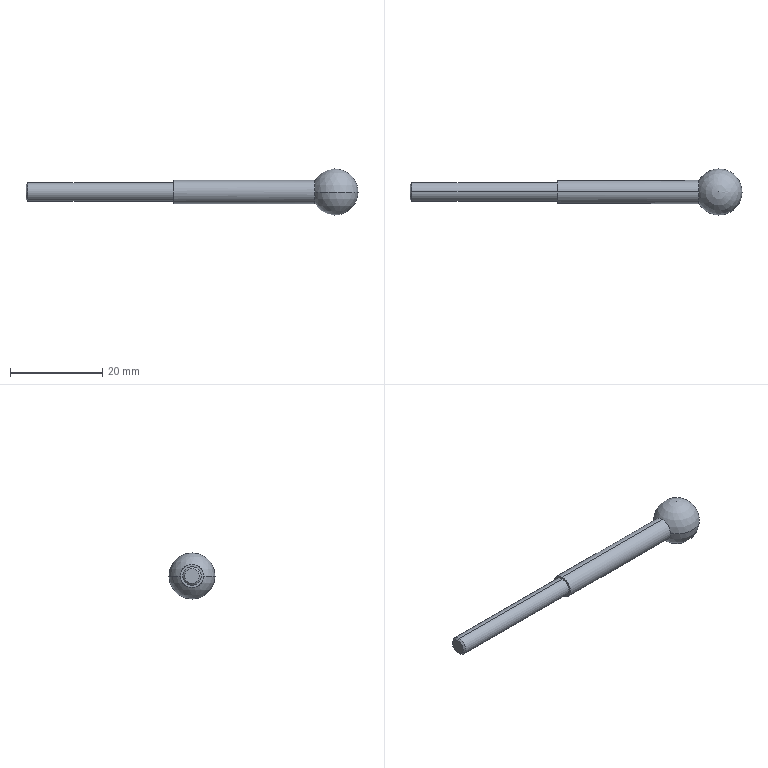Part | SolidWorks | features Extrusion 1, Revolution 1, StudWizard 1 | 1 solid | 10 faces | box 72 x 10 x 10 mm | volume 1520 mm3 | cylinder 4 | sphere 2 | cone 2 | plane 2 | commonest cylinder face diameters 4 x2 5 x2
STEP:
#1=CARTESIAN_POINT('',(67.,-5.,0.));
#2=VERTEX_POINT('',#1);
#3=CARTESIAN_POINT('',(67.,5.,0.));
#4=VERTEX_POINT('',#3);
#5=CARTESIAN_POINT('',(67.,0.,0.));
#6=DIRECTION('',(0.,0.,1.));
#7=DIRECTION('',(1.,0.,0.));
#8=AXIS2_PLACEMENT_3D('',#5,#6,#7);
#9=CIRCLE('',#8,5.);
#10=EDGE_CURVE('',#2,#4,#9,.T.);
#11=ORIENTED_EDGE('',*,*,#10,.F.);
#12=CARTESIAN_POINT('',(62.67,-2.5,0.));
#13=VERTEX_POINT('',#12);
#14=CARTESIAN_POINT('',(67.,0.,0.));
#15=DIRECTION('',(0.,0.,-1.));
#16=DIRECTION('',(-1.,0.,0.));
#17=AXIS2_PLACEMENT_3D('',#14,#15,#16);
#18=CIRCLE('',#17,5.);
#19=EDGE_CURVE('',#2,#13,#18,.T.);
#20=ORIENTED_EDGE('',*,*,#19,.T.);
#21=CARTESIAN_POINT('',(62.67,0.,-2.5));
#22=VERTEX_POINT('',#21);
#23=CARTESIAN_POINT('',(62.67,0.,0.));
#24=DIRECTION('',(1.,0.,0.));
#25=DIRECTION('',(0.,0.,-1.));
#26=AXIS2_PLACEMENT_3D('',#23,#24,#25);
#27=CIRCLE('',#26,2.5);
#28=EDGE_CURVE('',#13,#22,#27,.T.);
#29=ORIENTED_EDGE('',*,*,#28,.T.);
#30=CARTESIAN_POINT('',(62.67,2.5,0.));
#31=VERTEX_POINT('',#30);
#32=CARTESIAN_POINT('',(62.67,0.,0.));
#33=DIRECTION('',(1.,0.,0.));
#34=DIRECTION('',(0.,0.,-1.));
#35=AXIS2_PLACEMENT_3D('',#32,#33,#34);
#36=CIRCLE('',#35,2.5);
#37=EDGE_CURVE('',#22,#31,#36,.T.);
#38=ORIENTED_EDGE('',*,*,#37,.T.);
#39=CARTESIAN_POINT('',(67.,0.,0.));
#40=DIRECTION('',(0.,0.,-1.));
#41=DIRECTION('',(-1.,0.,0.));
#42=AXIS2_PLACEMENT_3D('',#39,#40,#41);
#43=CIRCLE('',#42,5.);
#44=EDGE_CURVE('',#31,#4,#43,.T.);
#45=ORIENTED_EDGE('',*,*,#44,.T.);
#46=EDGE_LOOP('',(#11,#20,#29,#38,#45));
#47=FACE_OUTER_BOUND('',#46,.T.);
#48=CARTESIAN_POINT('',(67.,0.,0.));
#49=DIRECTION('',(0.,0.,-1.));
#50=DIRECTION('',(1.,0.,0.));
#51=AXIS2_PLACEMENT_3D('',#48,#49,#50);
#52=SPHERICAL_SURFACE('',#51,5.);
#53=ADVANCED_FACE('',(#47),#52,.T.);
#54=CARTESIAN_POINT('',(0.,0.,-1.621));
#55=VERTEX_POINT('',#54);
#56=CARTESIAN_POINT('',(0.,0.,1.621));
#57=VERTEX_POINT('',#56);
#58=CARTESIAN_POINT('',(0.,0.,0.));
#59=DIRECTION('',(1.,0.,0.));
#60=DIRECTION('',(0.,0.,-1.));
#61=AXIS2_PLACEMENT_3D('',#58,#59,#60);
#62=CIRCLE('',#61,1.621);
#63=EDGE_CURVE('',#55,#57,#62,.T.);
#64=ORIENTED_EDGE('',*,*,#63,.T.);
#65=CARTESIAN_POINT('',(0.379,0.,2.));
#66=VERTEX_POINT('',#65);
#67=CARTESIAN_POINT('',(0.,0.,1.621));
#68=DIRECTION('',(0.7071,0.,0.7071));
#69=VECTOR('',#68,1000.);
#70=LINE('',#67,#69);
#71=EDGE_CURVE('',#57,#66,#70,.T.);
#72=ORIENTED_EDGE('',*,*,#71,.T.);
#73=CARTESIAN_POINT('',(0.379,0.,-2.));
#74=VERTEX_POINT('',#73);
#75=CARTESIAN_POINT('',(0.379,0.,0.));
#76=DIRECTION('',(1.,0.,0.));
#77=DIRECTION('',(0.,0.,-1.));
#78=AXIS2_PLACEMENT_3D('',#75,#76,#77);
#79=CIRCLE('',#78,2.);
#80=EDGE_CURVE('',#74,#66,#79,.T.);
#81=ORIENTED_EDGE('',*,*,#80,.F.);
#82=CARTESIAN_POINT('',(0.,0.,-1.621));
#83=DIRECTION('',(0.7071,0.,-0.7071));
#84=VECTOR('',#83,1000.);
#85=LINE('',#82,#84);
#86=EDGE_CURVE('',#55,#74,#85,.T.);
#87=ORIENTED_EDGE('',*,*,#86,.F.);
#88=EDGE_LOOP('',(#64,#72,#81,#87));
#89=FACE_OUTER_BOUND('',#88,.T.);
#90=CARTESIAN_POINT('',(0.,0.,0.));
#91=DIRECTION('',(1.,0.,0.));
#92=DIRECTION('',(0.,0.,-1.));
#93=AXIS2_PLACEMENT_3D('',#90,#91,#92);
#94=CONICAL_SURFACE('',#93,1.621,0.7854);
#95=ADVANCED_FACE('',(#89),#94,.T.);
#96=ORIENTED_EDGE('',*,*,#80,.T.);
#97=CARTESIAN_POINT('',(32.,0.,2.));
#98=VERTEX_POINT('',#97);
#99=CARTESIAN_POINT('',(0.,0.,2.));
#100=DIRECTION('',(1.,0.,0.));
#101=VECTOR('',#100,1000.);
#102=LINE('',#99,#101);
#103=EDGE_CURVE('',#66,#98,#102,.T.);
#104=ORIENTED_EDGE('',*,*,#103,.T.);
#105=CARTESIAN_POINT('',(32.,0.,-2.));
#106=VERTEX_POINT('',#105);
#107=CARTESIAN_POINT('',(32.,0.,0.));
#108=DIRECTION('',(1.,0.,0.));
#109=DIRECTION('',(0.,0.,-1.));
#110=AXIS2_PLACEMENT_3D('',#107,#108,#109);
#111=CIRCLE('',#110,2.);
#112=EDGE_CURVE('',#106,#98,#111,.T.);
#113=ORIENTED_EDGE('',*,*,#112,.F.);
#114=CARTESIAN_POINT('',(0.,0.,-2.));
#115=DIRECTION('',(1.,0.,0.));
#116=VECTOR('',#115,1000.);
#117=LINE('',#114,#116);
#118=EDGE_CURVE('',#74,#106,#117,.T.);
#119=ORIENTED_EDGE('',*,*,#118,.F.);
#120=EDGE_LOOP('',(#96,#104,#113,#119));
#121=FACE_OUTER_BOUND('',#120,.T.);
#122=CARTESIAN_POINT('',(0.,0.,0.));
#123=DIRECTION('',(1.,0.,0.));
#124=DIRECTION('',(0.,0.,-1.));
#125=AXIS2_PLACEMENT_3D('',#122,#123,#124);
#126=CYLINDRICAL_SURFACE('',#125,2.);
#127=ADVANCED_FACE('',(#121),#126,.T.);
#128=ORIENTED_EDGE('',*,*,#37,.F.);
#129=CARTESIAN_POINT('',(32.,0.,-2.5));
#130=VERTEX_POINT('',#129);
#131=CARTESIAN_POINT('',(67.,0.,-2.5));
#132=DIRECTION('',(-1.,0.,0.));
#133=VECTOR('',#132,1000.);
#134=LINE('',#131,#133);
#135=EDGE_CURVE('',#22,#130,#134,.T.);
#136=ORIENTED_EDGE('',*,*,#135,.T.);
#137=CARTESIAN_POINT('',(32.,0.,2.5));
#138=VERTEX_POINT('',#137);
#139=CARTESIAN_POINT('',(32.,0.,0.));
#140=DIRECTION('',(1.,0.,0.));
#141=DIRECTION('',(0.,0.,-1.));
#142=AXIS2_PLACEMENT_3D('',#139,#140,#141);
#143=CIRCLE('',#142,2.5);
#144=EDGE_CURVE('',#130,#138,#143,.T.);
#145=ORIENTED_EDGE('',*,*,#144,.T.);
#146=CARTESIAN_POINT('',(62.67,0.,2.5));
#147=VERTEX_POINT('',#146);
#148=CARTESIAN_POINT('',(67.,0.,2.5));
#149=DIRECTION('',(-1.,0.,0.));
#150=VECTOR('',#149,1000.);
#151=LINE('',#148,#150);
#152=EDGE_CURVE('',#147,#138,#151,.T.);
#153=ORIENTED_EDGE('',*,*,#152,.F.);
#154=CARTESIAN_POINT('',(62.67,0.,0.));
#155=DIRECTION('',(1.,0.,0.));
#156=DIRECTION('',(0.,0.,-1.));
#157=AXIS2_PLACEMENT_3D('',#154,#155,#156);
#158=CIRCLE('',#157,2.5);
#159=EDGE_CURVE('',#31,#147,#158,.T.);
#160=ORIENTED_EDGE('',*,*,#159,.F.);
#161=EDGE_LOOP('',(#128,#136,#145,#153,#160));
#162=FACE_OUTER_BOUND('',#161,.T.);
#163=CARTESIAN_POINT('',(67.,0.,0.));
#164=DIRECTION('',(-1.,0.,0.));
#165=DIRECTION('',(0.,0.,1.));
#166=AXIS2_PLACEMENT_3D('',#163,#164,#165);
#167=CYLINDRICAL_SURFACE('',#166,2.5);
#168=ADVANCED_FACE('',(#162),#167,.T.);
#169=ORIENTED_EDGE('',*,*,#135,.F.);
#170=ORIENTED_EDGE('',*,*,#28,.F.);
#171=CARTESIAN_POINT('',(62.67,0.,0.));
#172=DIRECTION('',(1.,0.,0.));
#173=DIRECTION('',(0.,0.,-1.));
#174=AXIS2_PLACEMENT_3D('',#171,#172,#173);
#175=CIRCLE('',#174,2.5);
#176=EDGE_CURVE('',#147,#13,#175,.T.);
#177=ORIENTED_EDGE('',*,*,#176,.F.);
#178=ORIENTED_EDGE('',*,*,#152,.T.);
#179=CARTESIAN_POINT('',(32.,0.,0.));
#180=DIRECTION('',(1.,0.,0.));
#181=DIRECTION('',(0.,0.,-1.));
#182=AXIS2_PLACEMENT_3D('',#179,#180,#181);
#183=CIRCLE('',#182,2.5);
#184=EDGE_CURVE('',#138,#130,#183,.T.);
#185=ORIENTED_EDGE('',*,*,#184,.T.);
#186=EDGE_LOOP('',(#169,#170,#177,#178,#185));
#187=FACE_OUTER_BOUND('',#186,.T.);
#188=CARTESIAN_POINT('',(67.,0.,0.));
#189=DIRECTION('',(-1.,0.,0.));
#190=DIRECTION('',(0.,0.,1.));
#191=AXIS2_PLACEMENT_3D('',#188,#189,#190);
#192=CYLINDRICAL_SURFACE('',#191,2.5);
#193=ADVANCED_FACE('',(#187),#192,.T.);
#194=ORIENTED_EDGE('',*,*,#103,.F.);
#195=CARTESIAN_POINT('',(0.379,0.,0.));
#196=DIRECTION('',(1.,0.,0.));
#197=DIRECTION('',(0.,0.,-1.));
#198=AXIS2_PLACEMENT_3D('',#195,#196,#197);
#199=CIRCLE('',#198,2.);
#200=EDGE_CURVE('',#66,#74,#199,.T.);
#201=ORIENTED_EDGE('',*,*,#200,.T.);
#202=ORIENTED_EDGE('',*,*,#118,.T.);
#203=CARTESIAN_POINT('',(32.,0.,0.));
#204=DIRECTION('',(1.,0.,0.));
#205=DIRECTION('',(0.,0.,-1.));
#206=AXIS2_PLACEMENT_3D('',#203,#204,#205);
#207=CIRCLE('',#206,2.);
#208=EDGE_CURVE('',#98,#106,#207,.T.);
#209=ORIENTED_EDGE('',*,*,#208,.F.);
#210=EDGE_LOOP('',(#194,#201,#202,#209));
#211=FACE_OUTER_BOUND('',#210,.T.);
#212=CARTESIAN_POINT('',(0.,0.,0.));
#213=DIRECTION('',(1.,0.,0.));
#214=DIRECTION('',(0.,0.,-1.));
#215=AXIS2_PLACEMENT_3D('',#212,#213,#214);
#216=CYLINDRICAL_SURFACE('',#215,2.);
#217=ADVANCED_FACE('',(#211),#216,.T.);
#218=ORIENTED_EDGE('',*,*,#184,.F.);
#219=ORIENTED_EDGE('',*,*,#144,.F.);
#220=EDGE_LOOP('',(#218,#219));
#221=FACE_OUTER_BOUND('',#220,.T.);
#222=ORIENTED_EDGE('',*,*,#112,.T.);
#223=ORIENTED_EDGE('',*,*,#208,.T.);
#224=EDGE_LOOP('',(#222,#223));
#225=FACE_BOUND('',#224,.T.);
#226=CARTESIAN_POINT('',(32.,2.,0.));
#227=DIRECTION('',(1.,0.,0.));
#228=DIRECTION('',(0.,0.,-1.));
#229=AXIS2_PLACEMENT_3D('',#226,#227,#228);
#230=PLANE('',#229);
#231=ADVANCED_FACE('',(#221,#225),#230,.F.);
#232=ORIENTED_EDGE('',*,*,#71,.F.);
#233=CARTESIAN_POINT('',(0.,0.,0.));
#234=DIRECTION('',(1.,0.,0.));
#235=DIRECTION('',(0.,0.,-1.));
#236=AXIS2_PLACEMENT_3D('',#233,#234,#235);
#237=CIRCLE('',#236,1.621);
#238=EDGE_CURVE('',#57,#55,#237,.T.);
#239=ORIENTED_EDGE('',*,*,#238,.T.);
#240=ORIENTED_EDGE('',*,*,#86,.T.);
#241=ORIENTED_EDGE('',*,*,#200,.F.);
#242=EDGE_LOOP('',(#232,#239,#240,#241));
#243=FACE_OUTER_BOUND('',#242,.T.);
#244=CARTESIAN_POINT('',(0.,0.,0.));
#245=DIRECTION('',(1.,0.,0.));
#246=DIRECTION('',(0.,0.,-1.));
#247=AXIS2_PLACEMENT_3D('',#244,#245,#246);
#248=CONICAL_SURFACE('',#247,1.621,0.7854);
#249=ADVANCED_FACE('',(#243),#248,.T.);
#250=ORIENTED_EDGE('',*,*,#63,.F.);
#251=ORIENTED_EDGE('',*,*,#238,.F.);
#252=EDGE_LOOP('',(#250,#251));
#253=FACE_OUTER_BOUND('',#252,.T.);
#254=CARTESIAN_POINT('',(0.,0.,0.));
#255=DIRECTION('',(1.,0.,0.));
#256=DIRECTION('',(0.,0.,-1.));
#257=AXIS2_PLACEMENT_3D('',#254,#255,#256);
#258=PLANE('',#257);
#259=ADVANCED_FACE('',(#253),#258,.F.);
#260=ORIENTED_EDGE('',*,*,#19,.F.);
#261=ORIENTED_EDGE('',*,*,#10,.T.);
#262=ORIENTED_EDGE('',*,*,#44,.F.);
#263=ORIENTED_EDGE('',*,*,#159,.T.);
#264=ORIENTED_EDGE('',*,*,#176,.T.);
#265=EDGE_LOOP('',(#260,#261,#262,#263,#264));
#266=FACE_OUTER_BOUND('',#265,.T.);
#267=CARTESIAN_POINT('',(67.,0.,0.));
#268=DIRECTION('',(0.,0.,-1.));
#269=DIRECTION('',(1.,0.,0.));
#270=AXIS2_PLACEMENT_3D('',#267,#268,#269);
#271=SPHERICAL_SURFACE('',#270,5.);
#272=ADVANCED_FACE('',(#266),#271,.T.);
#273=CLOSED_SHELL('',(#53,#95,#127,#168,#193,#217,#231,#249,#259,#272));
#274=MANIFOLD_SOLID_BREP('',#273);
#275=CARTESIAN_POINT('',(0.,0.,0.));
#276=DIRECTION('',(0.,0.,1.));
#277=DIRECTION('',(1.,0.,0.));
#278=AXIS2_PLACEMENT_3D('',#275,#276,#277);
#279=(LENGTH_UNIT()NAMED_UNIT(*)SI_UNIT(.MILLI.,.METRE.));
#280=UNCERTAINTY_MEASURE_WITH_UNIT(LENGTH_MEASURE(0.00001),#279,'','');
#281=(NAMED_UNIT(*)PLANE_ANGLE_UNIT()SI_UNIT($,.RADIAN.));
#282=(NAMED_UNIT(*)SI_UNIT($,.STERADIAN.)SOLID_ANGLE_UNIT());
#283=(GEOMETRIC_REPRESENTATION_CONTEXT(3)GLOBAL_UNCERTAINTY_ASSIGNED_CONTEXT((#280))GLOBAL_UNIT_ASSIGNED_CONTEXT((#279,#281,#282))REPRESENTATION_CONTEXT('',''));
#284=ADVANCED_BREP_SHAPE_REPRESENTATION('',(#274,#278),#283);